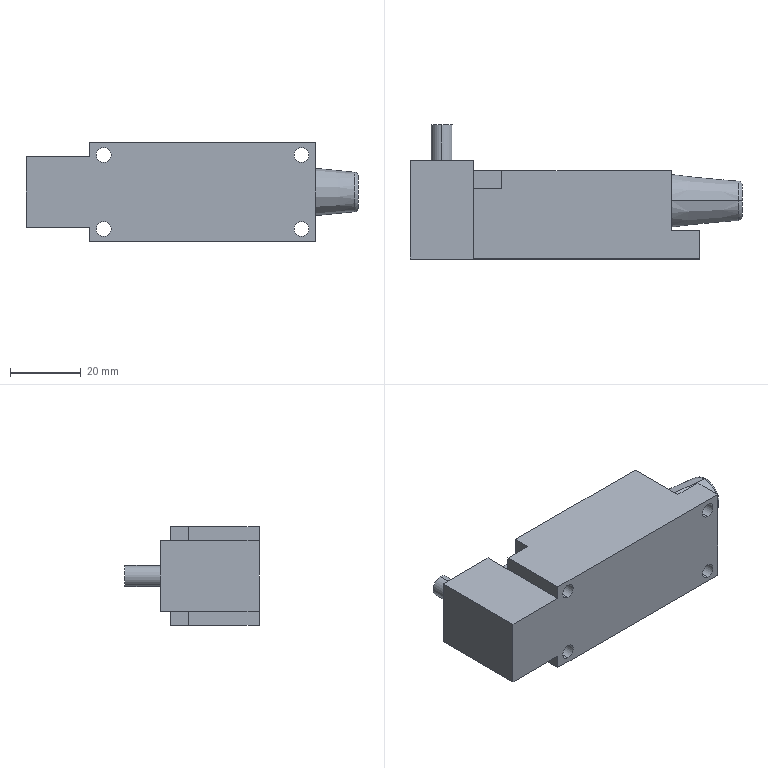Part | STEP file | switch | 1 solid | 36 faces | box 94 x 38 x 28 mm | volume 52689 mm3 | plane 22 | cylinder 10 | torus 2 | cone 2 | commonest cylinder face diameters 4.2 x8 6 x2